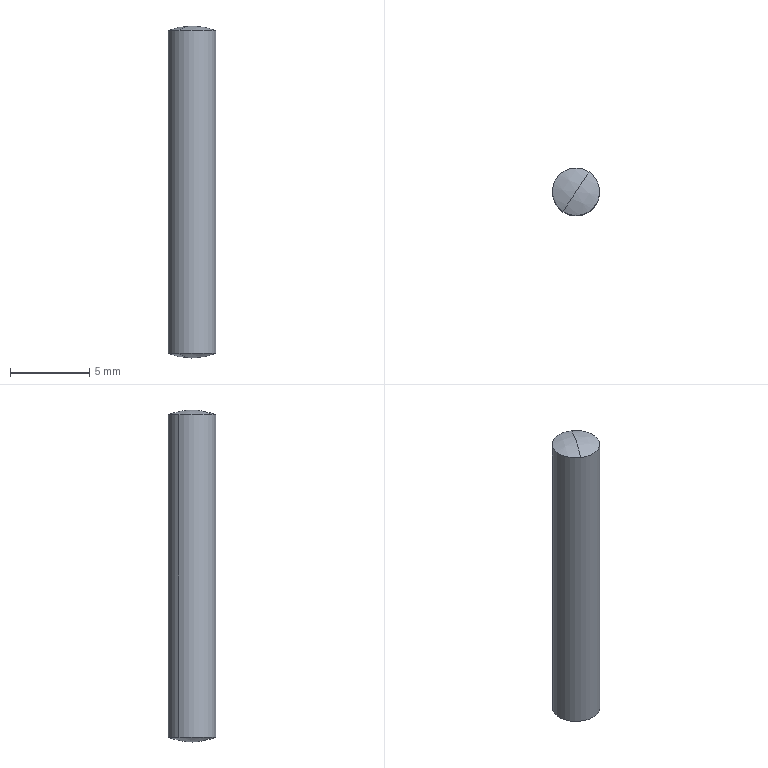Part | SolidWorks | features BaseBody 1 | 1 solid | 6 faces | box 3 x 3 x 21 mm | volume 146.403 mm3 | sphere 4 | cylinder 2 | commonest cylinder face diameters 3 x2
STEP:
#1=CARTESIAN_POINT('',(257.226,98.352,-5.692));
#2=VERTEX_POINT('',#1);
#3=CARTESIAN_POINT('',(257.652,96.274,-5.692));
#4=VERTEX_POINT('',#3);
#5=CARTESIAN_POINT('',(256.4,97.1,-5.692));
#6=DIRECTION('',(0.,0.,-1.));
#7=DIRECTION('',(-0.8349,0.5504,0.));
#8=AXIS2_PLACEMENT_3D('',#5,#6,#7);
#9=CIRCLE('',#8,1.5);
#10=EDGE_CURVE('',#2,#4,#9,.T.);
#11=ORIENTED_EDGE('',*,*,#10,.T.);
#12=CARTESIAN_POINT('',(257.652,96.274,-26.108));
#13=VERTEX_POINT('',#12);
#14=CARTESIAN_POINT('',(257.652,96.274,-26.4));
#15=DIRECTION('',(0.,0.,-1.));
#16=VECTOR('',#15,1000.);
#17=LINE('',#14,#16);
#18=EDGE_CURVE('',#4,#13,#17,.T.);
#19=ORIENTED_EDGE('',*,*,#18,.T.);
#20=CARTESIAN_POINT('',(257.226,98.352,-26.108));
#21=VERTEX_POINT('',#20);
#22=CARTESIAN_POINT('',(256.4,97.1,-26.108));
#23=DIRECTION('',(0.,0.,-1.));
#24=DIRECTION('',(-0.8349,0.5504,0.));
#25=AXIS2_PLACEMENT_3D('',#22,#23,#24);
#26=CIRCLE('',#25,1.5);
#27=EDGE_CURVE('',#21,#13,#26,.T.);
#28=ORIENTED_EDGE('',*,*,#27,.F.);
#29=CARTESIAN_POINT('',(255.148,97.926,-26.108));
#30=VERTEX_POINT('',#29);
#31=CARTESIAN_POINT('',(256.4,97.1,-26.108));
#32=DIRECTION('',(0.,0.,-1.));
#33=DIRECTION('',(-0.8349,0.5504,0.));
#34=AXIS2_PLACEMENT_3D('',#31,#32,#33);
#35=CIRCLE('',#34,1.5);
#36=EDGE_CURVE('',#30,#21,#35,.T.);
#37=ORIENTED_EDGE('',*,*,#36,.F.);
#38=CARTESIAN_POINT('',(255.148,97.926,-5.692));
#39=VERTEX_POINT('',#38);
#40=CARTESIAN_POINT('',(255.148,97.926,-26.4));
#41=DIRECTION('',(0.,0.,-1.));
#42=VECTOR('',#41,1000.);
#43=LINE('',#40,#42);
#44=EDGE_CURVE('',#39,#30,#43,.T.);
#45=ORIENTED_EDGE('',*,*,#44,.F.);
#46=CARTESIAN_POINT('',(256.4,97.1,-5.692));
#47=DIRECTION('',(0.,0.,-1.));
#48=DIRECTION('',(-0.8349,0.5504,0.));
#49=AXIS2_PLACEMENT_3D('',#46,#47,#48);
#50=CIRCLE('',#49,1.5);
#51=EDGE_CURVE('',#39,#2,#50,.T.);
#52=ORIENTED_EDGE('',*,*,#51,.T.);
#53=EDGE_LOOP('',(#11,#19,#28,#37,#45,#52));
#54=FACE_OUTER_BOUND('',#53,.T.);
#55=CARTESIAN_POINT('',(256.4,97.1,-26.4));
#56=DIRECTION('',(0.,0.,-1.));
#57=DIRECTION('',(-0.8349,0.5504,0.));
#58=AXIS2_PLACEMENT_3D('',#55,#56,#57);
#59=CYLINDRICAL_SURFACE('',#58,1.5);
#60=ADVANCED_FACE('',(#54),#59,.T.);
#61=CARTESIAN_POINT('',(256.4,97.1,-5.4));
#62=VERTEX_POINT('',#61);
#63=CARTESIAN_POINT('',(256.4,97.1,-9.4));
#64=DIRECTION('',(-0.8349,0.5504,0.));
#65=DIRECTION('',(-0.5504,-0.8349,0.));
#66=AXIS2_PLACEMENT_3D('',#63,#64,#65);
#67=CIRCLE('',#66,4.);
#68=EDGE_CURVE('',#62,#2,#67,.T.);
#69=ORIENTED_EDGE('',*,*,#68,.F.);
#70=CARTESIAN_POINT('',(255.574,95.848,-5.692));
#71=VERTEX_POINT('',#70);
#72=CARTESIAN_POINT('',(256.4,97.1,-9.4));
#73=DIRECTION('',(0.8349,-0.5504,0.));
#74=DIRECTION('',(0.5504,0.8349,0.));
#75=AXIS2_PLACEMENT_3D('',#72,#73,#74);
#76=CIRCLE('',#75,4.);
#77=EDGE_CURVE('',#62,#71,#76,.T.);
#78=ORIENTED_EDGE('',*,*,#77,.T.);
#79=CARTESIAN_POINT('',(256.4,97.1,-5.692));
#80=DIRECTION('',(0.,0.,-1.));
#81=DIRECTION('',(-0.8349,0.5504,0.));
#82=AXIS2_PLACEMENT_3D('',#79,#80,#81);
#83=CIRCLE('',#82,1.5);
#84=EDGE_CURVE('',#4,#71,#83,.T.);
#85=ORIENTED_EDGE('',*,*,#84,.F.);
#86=ORIENTED_EDGE('',*,*,#10,.F.);
#87=EDGE_LOOP('',(#69,#78,#85,#86));
#88=FACE_OUTER_BOUND('',#87,.T.);
#89=CARTESIAN_POINT('',(256.4,97.1,-9.4));
#90=DIRECTION('',(0.8349,-0.5504,0.));
#91=DIRECTION('',(0.5504,0.8349,0.));
#92=AXIS2_PLACEMENT_3D('',#89,#90,#91);
#93=SPHERICAL_SURFACE('',#92,4.);
#94=ADVANCED_FACE('',(#88),#93,.T.);
#95=ORIENTED_EDGE('',*,*,#27,.T.);
#96=CARTESIAN_POINT('',(255.574,95.848,-26.108));
#97=VERTEX_POINT('',#96);
#98=CARTESIAN_POINT('',(256.4,97.1,-26.108));
#99=DIRECTION('',(0.,0.,-1.));
#100=DIRECTION('',(-0.8349,0.5504,0.));
#101=AXIS2_PLACEMENT_3D('',#98,#99,#100);
#102=CIRCLE('',#101,1.5);
#103=EDGE_CURVE('',#13,#97,#102,.T.);
#104=ORIENTED_EDGE('',*,*,#103,.T.);
#105=CARTESIAN_POINT('',(256.4,97.1,-26.4));
#106=VERTEX_POINT('',#105);
#107=CARTESIAN_POINT('',(256.4,97.1,-22.4));
#108=DIRECTION('',(0.8349,-0.5504,0.));
#109=DIRECTION('',(0.5504,0.8349,0.));
#110=AXIS2_PLACEMENT_3D('',#107,#108,#109);
#111=CIRCLE('',#110,4.);
#112=EDGE_CURVE('',#97,#106,#111,.T.);
#113=ORIENTED_EDGE('',*,*,#112,.T.);
#114=CARTESIAN_POINT('',(256.4,97.1,-22.4));
#115=DIRECTION('',(-0.8349,0.5504,0.));
#116=DIRECTION('',(-0.5504,-0.8349,0.));
#117=AXIS2_PLACEMENT_3D('',#114,#115,#116);
#118=CIRCLE('',#117,4.);
#119=EDGE_CURVE('',#21,#106,#118,.T.);
#120=ORIENTED_EDGE('',*,*,#119,.F.);
#121=EDGE_LOOP('',(#95,#104,#113,#120));
#122=FACE_OUTER_BOUND('',#121,.T.);
#123=CARTESIAN_POINT('',(256.4,97.1,-22.4));
#124=DIRECTION('',(0.8349,-0.5504,0.));
#125=DIRECTION('',(0.5504,0.8349,0.));
#126=AXIS2_PLACEMENT_3D('',#123,#124,#125);
#127=SPHERICAL_SURFACE('',#126,4.);
#128=ADVANCED_FACE('',(#122),#127,.T.);
#129=ORIENTED_EDGE('',*,*,#112,.F.);
#130=CARTESIAN_POINT('',(256.4,97.1,-26.108));
#131=DIRECTION('',(0.,0.,-1.));
#132=DIRECTION('',(-0.8349,0.5504,0.));
#133=AXIS2_PLACEMENT_3D('',#130,#131,#132);
#134=CIRCLE('',#133,1.5);
#135=EDGE_CURVE('',#97,#30,#134,.T.);
#136=ORIENTED_EDGE('',*,*,#135,.T.);
#137=ORIENTED_EDGE('',*,*,#36,.T.);
#138=ORIENTED_EDGE('',*,*,#119,.T.);
#139=EDGE_LOOP('',(#129,#136,#137,#138));
#140=FACE_OUTER_BOUND('',#139,.T.);
#141=CARTESIAN_POINT('',(256.4,97.1,-22.4));
#142=DIRECTION('',(0.8349,-0.5504,0.));
#143=DIRECTION('',(0.5504,0.8349,0.));
#144=AXIS2_PLACEMENT_3D('',#141,#142,#143);
#145=SPHERICAL_SURFACE('',#144,4.);
#146=ADVANCED_FACE('',(#140),#145,.T.);
#147=ORIENTED_EDGE('',*,*,#77,.F.);
#148=ORIENTED_EDGE('',*,*,#68,.T.);
#149=ORIENTED_EDGE('',*,*,#51,.F.);
#150=CARTESIAN_POINT('',(256.4,97.1,-5.692));
#151=DIRECTION('',(0.,0.,-1.));
#152=DIRECTION('',(-0.8349,0.5504,0.));
#153=AXIS2_PLACEMENT_3D('',#150,#151,#152);
#154=CIRCLE('',#153,1.5);
#155=EDGE_CURVE('',#71,#39,#154,.T.);
#156=ORIENTED_EDGE('',*,*,#155,.F.);
#157=EDGE_LOOP('',(#147,#148,#149,#156));
#158=FACE_OUTER_BOUND('',#157,.T.);
#159=CARTESIAN_POINT('',(256.4,97.1,-9.4));
#160=DIRECTION('',(0.8349,-0.5504,0.));
#161=DIRECTION('',(0.5504,0.8349,0.));
#162=AXIS2_PLACEMENT_3D('',#159,#160,#161);
#163=SPHERICAL_SURFACE('',#162,4.);
#164=ADVANCED_FACE('',(#158),#163,.T.);
#165=ORIENTED_EDGE('',*,*,#18,.F.);
#166=ORIENTED_EDGE('',*,*,#84,.T.);
#167=ORIENTED_EDGE('',*,*,#155,.T.);
#168=ORIENTED_EDGE('',*,*,#44,.T.);
#169=ORIENTED_EDGE('',*,*,#135,.F.);
#170=ORIENTED_EDGE('',*,*,#103,.F.);
#171=EDGE_LOOP('',(#165,#166,#167,#168,#169,#170));
#172=FACE_OUTER_BOUND('',#171,.T.);
#173=CARTESIAN_POINT('',(256.4,97.1,-26.4));
#174=DIRECTION('',(0.,0.,-1.));
#175=DIRECTION('',(-0.8349,0.5504,0.));
#176=AXIS2_PLACEMENT_3D('',#173,#174,#175);
#177=CYLINDRICAL_SURFACE('',#176,1.5);
#178=ADVANCED_FACE('',(#172),#177,.T.);
#179=CLOSED_SHELL('',(#60,#94,#128,#146,#164,#178));
#180=MANIFOLD_SOLID_BREP('',#179);
#181=CARTESIAN_POINT('',(0.,0.,0.));
#182=DIRECTION('',(0.,0.,1.));
#183=DIRECTION('',(1.,0.,0.));
#184=AXIS2_PLACEMENT_3D('',#181,#182,#183);
#185=(LENGTH_UNIT()NAMED_UNIT(*)SI_UNIT(.MILLI.,.METRE.));
#186=UNCERTAINTY_MEASURE_WITH_UNIT(LENGTH_MEASURE(0.00001),#185,'','');
#187=(NAMED_UNIT(*)PLANE_ANGLE_UNIT()SI_UNIT($,.RADIAN.));
#188=(NAMED_UNIT(*)SI_UNIT($,.STERADIAN.)SOLID_ANGLE_UNIT());
#189=(GEOMETRIC_REPRESENTATION_CONTEXT(3)GLOBAL_UNCERTAINTY_ASSIGNED_CONTEXT((#186))GLOBAL_UNIT_ASSIGNED_CONTEXT((#185,#187,#188))REPRESENTATION_CONTEXT('',''));
#190=ADVANCED_BREP_SHAPE_REPRESENTATION('',(#180,#184),#189);